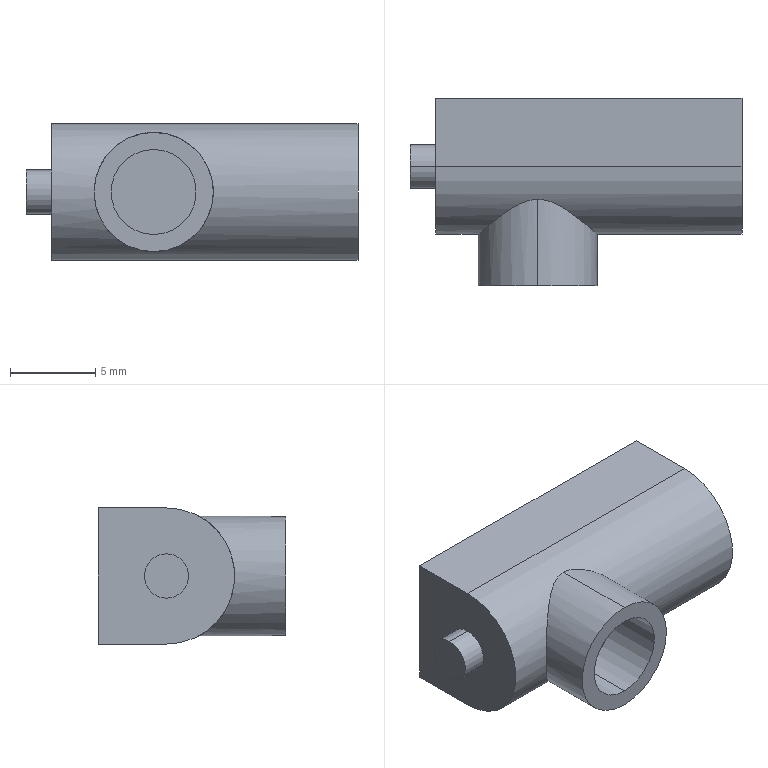Part | STEP file | _AF30-A(0)_DRAIN | 1 solid | 15 faces | box 19.5 x 11 x 8 mm | volume 1100 mm3 | plane 8 | cylinder 7 | commonest cylinder face diameters 2.6 x2 5 x2 7 x2 8 x1
STEP:
#1=CARTESIAN_POINT('',(-3.,-5.936,3.5));
#2=VERTEX_POINT('',#1);
#3=CARTESIAN_POINT('',(-3.,-5.936,-3.5));
#4=VERTEX_POINT('',#3);
#5=CARTESIAN_POINT('',(-3.,-5.936,3.5));
#6=CARTESIAN_POINT('',(-2.749,-5.936,3.5));
#7=CARTESIAN_POINT('',(-2.506,-5.987,3.473));
#8=CARTESIAN_POINT('',(-2.044,-6.149,3.375));
#9=CARTESIAN_POINT('',(-1.832,-6.255,3.307));
#10=CARTESIAN_POINT('',(-1.429,-6.488,3.135));
#11=CARTESIAN_POINT('',(-1.239,-6.614,3.032));
#12=CARTESIAN_POINT('',(-0.8863,-6.864,2.798));
#13=CARTESIAN_POINT('',(-0.7211,-6.989,2.665));
#14=CARTESIAN_POINT('',(-0.4112,-7.232,2.365));
#15=CARTESIAN_POINT('',(-0.2667,-7.349,2.197));
#16=CARTESIAN_POINT('',(-0.01033,-7.561,1.833));
#17=CARTESIAN_POINT('',(0.1034,-7.658,1.635));
#18=CARTESIAN_POINT('',(0.2947,-7.821,1.204));
#19=CARTESIAN_POINT('',(0.3694,-7.886,0.9781));
#20=CARTESIAN_POINT('',(0.4467,-7.953,0.6204));
#21=CARTESIAN_POINT('',(0.4667,-7.971,0.4973));
#22=CARTESIAN_POINT('',(0.4931,-7.994,0.2519));
#23=CARTESIAN_POINT('',(0.4998,-8.,0.1289));
#24=CARTESIAN_POINT('',(0.5004,-8.,-0.2405));
#25=CARTESIAN_POINT('',(0.4739,-7.977,-0.4912));
#26=CARTESIAN_POINT('',(0.3724,-7.889,-0.9675));
#27=CARTESIAN_POINT('',(0.2971,-7.823,-1.198));
#28=CARTESIAN_POINT('',(0.01254,-7.58,-1.843));
#29=CARTESIAN_POINT('',(-0.2533,-7.355,-2.211));
#30=CARTESIAN_POINT('',(-0.7151,-6.994,-2.66));
#31=CARTESIAN_POINT('',(-0.8806,-6.868,-2.794));
#32=CARTESIAN_POINT('',(-1.238,-6.615,-3.032));
#33=CARTESIAN_POINT('',(-1.426,-6.49,-3.134));
#34=CARTESIAN_POINT('',(-1.726,-6.316,-3.262));
#35=CARTESIAN_POINT('',(-1.83,-6.261,-3.301));
#36=CARTESIAN_POINT('',(-2.045,-6.157,-3.369));
#37=CARTESIAN_POINT('',(-2.158,-6.109,-3.399));
#38=CARTESIAN_POINT('',(-2.387,-6.028,-3.448));
#39=CARTESIAN_POINT('',(-2.505,-5.995,-3.467));
#40=CARTESIAN_POINT('',(-2.749,-5.949,-3.493));
#41=CARTESIAN_POINT('',(-2.874,-5.936,-3.5));
#42=CARTESIAN_POINT('',(-3.,-5.936,-3.5));
#43=B_SPLINE_CURVE_WITH_KNOTS('',3,(#5,#6,#7,#8,#9,#10,#11,#12,#13,#14,#15,#16,#17,#18,#19,#20,#21,#22,#23,#24,#25,#26,#27,#28,#29,#30,#31,#32,#33,#34,#35,#36,#37,#38,#39,#40,#41,#42),.UNSPECIFIED.,.F.,.F.,(4,2,2,2,2,2,2,2,2,2,2,2,2,2,2,2,2,2,4),(0.01185,0.0126,0.01334,0.01408,0.01482,0.01556,0.0163,0.01704,0.01741,0.01778,0.01852,0.01927,0.02075,0.02149,0.02223,0.0226,0.02297,0.02334,0.02371),.UNSPECIFIED.);
#44=EDGE_CURVE('',#2,#4,#43,.T.);
#45=ORIENTED_EDGE('',*,*,#44,.F.);
#46=CARTESIAN_POINT('',(-3.,-11.,3.5));
#47=VERTEX_POINT('',#46);
#48=CARTESIAN_POINT('',(-3.,0.,3.5));
#49=DIRECTION('',(0.,-1.,0.));
#50=VECTOR('',#49,1000.);
#51=LINE('',#48,#50);
#52=EDGE_CURVE('',#2,#47,#51,.T.);
#53=ORIENTED_EDGE('',*,*,#52,.T.);
#54=CARTESIAN_POINT('',(-3.,-11.,-3.5));
#55=VERTEX_POINT('',#54);
#56=CARTESIAN_POINT('',(-3.,-11.,0.));
#57=DIRECTION('',(0.,1.,0.));
#58=DIRECTION('',(0.,0.,-1.));
#59=AXIS2_PLACEMENT_3D('',#56,#57,#58);
#60=CIRCLE('',#59,3.5);
#61=EDGE_CURVE('',#47,#55,#60,.T.);
#62=ORIENTED_EDGE('',*,*,#61,.T.);
#63=CARTESIAN_POINT('',(-3.,0.,-3.5));
#64=DIRECTION('',(0.,-1.,0.));
#65=VECTOR('',#64,1000.);
#66=LINE('',#63,#65);
#67=EDGE_CURVE('',#4,#55,#66,.T.);
#68=ORIENTED_EDGE('',*,*,#67,.F.);
#69=EDGE_LOOP('',(#45,#53,#62,#68));
#70=FACE_OUTER_BOUND('',#69,.T.);
#71=CARTESIAN_POINT('',(-3.,0.,0.));
#72=DIRECTION('',(0.,-1.,0.));
#73=DIRECTION('',(0.,0.,-1.));
#74=AXIS2_PLACEMENT_3D('',#71,#72,#73);
#75=CYLINDRICAL_SURFACE('',#74,3.5);
#76=ADVANCED_FACE('',(#70),#75,.T.);
#77=CARTESIAN_POINT('',(-10.5,-4.,-1.3));
#78=VERTEX_POINT('',#77);
#79=CARTESIAN_POINT('',(-10.5,-4.,1.3));
#80=VERTEX_POINT('',#79);
#81=CARTESIAN_POINT('',(-10.5,-4.,0.));
#82=DIRECTION('',(1.,0.,0.));
#83=DIRECTION('',(0.,0.,-1.));
#84=AXIS2_PLACEMENT_3D('',#81,#82,#83);
#85=CIRCLE('',#84,1.3);
#86=EDGE_CURVE('',#78,#80,#85,.T.);
#87=ORIENTED_EDGE('',*,*,#86,.T.);
#88=CARTESIAN_POINT('',(-9.,-4.,1.3));
#89=VERTEX_POINT('',#88);
#90=CARTESIAN_POINT('',(-10.5,-4.,1.3));
#91=DIRECTION('',(1.,0.,0.));
#92=VECTOR('',#91,1000.);
#93=LINE('',#90,#92);
#94=EDGE_CURVE('',#80,#89,#93,.T.);
#95=ORIENTED_EDGE('',*,*,#94,.T.);
#96=CARTESIAN_POINT('',(-9.,-4.,-1.3));
#97=VERTEX_POINT('',#96);
#98=CARTESIAN_POINT('',(-9.,-4.,0.));
#99=DIRECTION('',(-1.,0.,0.));
#100=DIRECTION('',(0.,0.,-1.));
#101=AXIS2_PLACEMENT_3D('',#98,#99,#100);
#102=CIRCLE('',#101,1.3);
#103=EDGE_CURVE('',#89,#97,#102,.T.);
#104=ORIENTED_EDGE('',*,*,#103,.T.);
#105=CARTESIAN_POINT('',(-10.5,-4.,-1.3));
#106=DIRECTION('',(1.,0.,0.));
#107=VECTOR('',#106,1000.);
#108=LINE('',#105,#107);
#109=EDGE_CURVE('',#78,#97,#108,.T.);
#110=ORIENTED_EDGE('',*,*,#109,.F.);
#111=EDGE_LOOP('',(#87,#95,#104,#110));
#112=FACE_OUTER_BOUND('',#111,.T.);
#113=CARTESIAN_POINT('',(-10.5,-4.,0.));
#114=DIRECTION('',(1.,0.,0.));
#115=DIRECTION('',(0.,0.,-1.));
#116=AXIS2_PLACEMENT_3D('',#113,#114,#115);
#117=CYLINDRICAL_SURFACE('',#116,1.3);
#118=ADVANCED_FACE('',(#112),#117,.T.);
#119=CARTESIAN_POINT('',(-3.,-11.,2.5));
#120=VERTEX_POINT('',#119);
#121=CARTESIAN_POINT('',(-3.,-11.,-2.5));
#122=VERTEX_POINT('',#121);
#123=CARTESIAN_POINT('',(-3.,-11.,0.));
#124=DIRECTION('',(0.,-1.,0.));
#125=DIRECTION('',(0.,0.,1.));
#126=AXIS2_PLACEMENT_3D('',#123,#124,#125);
#127=CIRCLE('',#126,2.5);
#128=EDGE_CURVE('',#120,#122,#127,.T.);
#129=ORIENTED_EDGE('',*,*,#128,.T.);
#130=CARTESIAN_POINT('',(-3.,-7.5,-2.5));
#131=VERTEX_POINT('',#130);
#132=CARTESIAN_POINT('',(-3.,-7.5,-2.5));
#133=DIRECTION('',(0.,1.,0.));
#134=VECTOR('',#133,1000.);
#135=LINE('',#132,#134);
#136=EDGE_CURVE('',#122,#131,#135,.T.);
#137=ORIENTED_EDGE('',*,*,#136,.T.);
#138=CARTESIAN_POINT('',(-3.,-7.5,2.5));
#139=VERTEX_POINT('',#138);
#140=CARTESIAN_POINT('',(-3.,-7.5,0.));
#141=DIRECTION('',(0.,-1.,0.));
#142=DIRECTION('',(0.,0.,1.));
#143=AXIS2_PLACEMENT_3D('',#140,#141,#142);
#144=CIRCLE('',#143,2.5);
#145=EDGE_CURVE('',#139,#131,#144,.T.);
#146=ORIENTED_EDGE('',*,*,#145,.F.);
#147=CARTESIAN_POINT('',(-3.,-7.5,2.5));
#148=DIRECTION('',(0.,1.,0.));
#149=VECTOR('',#148,1000.);
#150=LINE('',#147,#149);
#151=EDGE_CURVE('',#120,#139,#150,.T.);
#152=ORIENTED_EDGE('',*,*,#151,.F.);
#153=EDGE_LOOP('',(#129,#137,#146,#152));
#154=FACE_OUTER_BOUND('',#153,.T.);
#155=CARTESIAN_POINT('',(-3.,-7.5,0.));
#156=DIRECTION('',(0.,1.,0.));
#157=DIRECTION('',(0.,0.,1.));
#158=AXIS2_PLACEMENT_3D('',#155,#156,#157);
#159=CYLINDRICAL_SURFACE('',#158,2.5);
#160=ADVANCED_FACE('',(#154),#159,.F.);
#161=CARTESIAN_POINT('',(-9.,-4.,4.));
#162=VERTEX_POINT('',#161);
#163=CARTESIAN_POINT('',(-9.,-4.,-4.));
#164=VERTEX_POINT('',#163);
#165=CARTESIAN_POINT('',(-9.,-4.,0.));
#166=DIRECTION('',(1.,0.,0.));
#167=DIRECTION('',(0.,0.,-1.));
#168=AXIS2_PLACEMENT_3D('',#165,#166,#167);
#169=CIRCLE('',#168,4.);
#170=EDGE_CURVE('',#162,#164,#169,.T.);
#171=ORIENTED_EDGE('',*,*,#170,.T.);
#172=CARTESIAN_POINT('',(9.,-4.,-4.));
#173=VERTEX_POINT('',#172);
#174=CARTESIAN_POINT('',(9.,-4.,-4.));
#175=DIRECTION('',(1.,0.,0.));
#176=VECTOR('',#175,1000.);
#177=LINE('',#174,#176);
#178=EDGE_CURVE('',#164,#173,#177,.T.);
#179=ORIENTED_EDGE('',*,*,#178,.T.);
#180=CARTESIAN_POINT('',(9.,-4.,4.));
#181=VERTEX_POINT('',#180);
#182=CARTESIAN_POINT('',(9.,-4.,0.));
#183=DIRECTION('',(-1.,0.,0.));
#184=DIRECTION('',(0.,0.,-1.));
#185=AXIS2_PLACEMENT_3D('',#182,#183,#184);
#186=CIRCLE('',#185,4.);
#187=EDGE_CURVE('',#173,#181,#186,.T.);
#188=ORIENTED_EDGE('',*,*,#187,.T.);
#189=CARTESIAN_POINT('',(9.,-4.,4.));
#190=DIRECTION('',(-1.,0.,0.));
#191=VECTOR('',#190,1000.);
#192=LINE('',#189,#191);
#193=EDGE_CURVE('',#181,#162,#192,.T.);
#194=ORIENTED_EDGE('',*,*,#193,.T.);
#195=EDGE_LOOP('',(#171,#179,#188,#194));
#196=FACE_OUTER_BOUND('',#195,.T.);
#197=CARTESIAN_POINT('',(-3.,-5.936,-3.5));
#198=CARTESIAN_POINT('',(-3.251,-5.936,-3.5));
#199=CARTESIAN_POINT('',(-3.494,-5.987,-3.473));
#200=CARTESIAN_POINT('',(-3.956,-6.149,-3.375));
#201=CARTESIAN_POINT('',(-4.168,-6.255,-3.307));
#202=CARTESIAN_POINT('',(-4.571,-6.488,-3.135));
#203=CARTESIAN_POINT('',(-4.761,-6.614,-3.032));
#204=CARTESIAN_POINT('',(-5.114,-6.864,-2.798));
#205=CARTESIAN_POINT('',(-5.279,-6.989,-2.665));
#206=CARTESIAN_POINT('',(-5.589,-7.232,-2.365));
#207=CARTESIAN_POINT('',(-5.733,-7.349,-2.197));
#208=CARTESIAN_POINT('',(-5.99,-7.561,-1.833));
#209=CARTESIAN_POINT('',(-6.103,-7.658,-1.635));
#210=CARTESIAN_POINT('',(-6.295,-7.821,-1.204));
#211=CARTESIAN_POINT('',(-6.369,-7.886,-0.9781));
#212=CARTESIAN_POINT('',(-6.447,-7.953,-0.6204));
#213=CARTESIAN_POINT('',(-6.467,-7.971,-0.4973));
#214=CARTESIAN_POINT('',(-6.493,-7.994,-0.2519));
#215=CARTESIAN_POINT('',(-6.5,-8.,-0.1289));
#216=CARTESIAN_POINT('',(-6.5,-8.,0.2405));
#217=CARTESIAN_POINT('',(-6.474,-7.977,0.4912));
#218=CARTESIAN_POINT('',(-6.372,-7.889,0.9675));
#219=CARTESIAN_POINT('',(-6.297,-7.823,1.198));
#220=CARTESIAN_POINT('',(-6.013,-7.58,1.843));
#221=CARTESIAN_POINT('',(-5.747,-7.355,2.211));
#222=CARTESIAN_POINT('',(-5.285,-6.994,2.66));
#223=CARTESIAN_POINT('',(-5.119,-6.868,2.794));
#224=CARTESIAN_POINT('',(-4.762,-6.615,3.032));
#225=CARTESIAN_POINT('',(-4.574,-6.49,3.134));
#226=CARTESIAN_POINT('',(-4.274,-6.316,3.262));
#227=CARTESIAN_POINT('',(-4.17,-6.261,3.301));
#228=CARTESIAN_POINT('',(-3.955,-6.157,3.369));
#229=CARTESIAN_POINT('',(-3.842,-6.109,3.399));
#230=CARTESIAN_POINT('',(-3.613,-6.028,3.448));
#231=CARTESIAN_POINT('',(-3.495,-5.995,3.467));
#232=CARTESIAN_POINT('',(-3.251,-5.949,3.493));
#233=CARTESIAN_POINT('',(-3.126,-5.936,3.5));
#234=CARTESIAN_POINT('',(-3.,-5.936,3.5));
#235=B_SPLINE_CURVE_WITH_KNOTS('',3,(#197,#198,#199,#200,#201,#202,#203,#204,#205,#206,#207,#208,#209,#210,#211,#212,#213,#214,#215,#216,#217,#218,#219,#220,#221,#222,#223,#224,#225,#226,#227,#228,#229,#230,#231,#232,#233,#234),.UNSPECIFIED.,.F.,.F.,(4,2,2,2,2,2,2,2,2,2,2,2,2,2,2,2,2,2,4),(0.,0.0007409,0.001482,0.002223,0.002964,0.003705,0.004445,0.005186,0.005557,0.005927,0.006668,0.007409,0.008891,0.009632,0.01037,0.01074,0.01111,0.01148,0.01185),.UNSPECIFIED.);
#236=EDGE_CURVE('',#4,#2,#235,.T.);
#237=ORIENTED_EDGE('',*,*,#236,.T.);
#238=ORIENTED_EDGE('',*,*,#44,.T.);
#239=EDGE_LOOP('',(#237,#238));
#240=FACE_BOUND('',#239,.T.);
#241=CARTESIAN_POINT('',(9.,-4.,0.));
#242=DIRECTION('',(1.,0.,0.));
#243=DIRECTION('',(0.,0.,-1.));
#244=AXIS2_PLACEMENT_3D('',#241,#242,#243);
#245=CYLINDRICAL_SURFACE('',#244,4.);
#246=ADVANCED_FACE('',(#196,#240),#245,.T.);
#247=CARTESIAN_POINT('',(9.,0.,-4.));
#248=VERTEX_POINT('',#247);
#249=CARTESIAN_POINT('',(9.,-4.,-4.));
#250=DIRECTION('',(0.,1.,0.));
#251=VECTOR('',#250,1000.);
#252=LINE('',#249,#251);
#253=EDGE_CURVE('',#173,#248,#252,.T.);
#254=ORIENTED_EDGE('',*,*,#253,.F.);
#255=ORIENTED_EDGE('',*,*,#178,.F.);
#256=CARTESIAN_POINT('',(-9.,0.,-4.));
#257=VERTEX_POINT('',#256);
#258=CARTESIAN_POINT('',(-9.,-4.,-4.));
#259=DIRECTION('',(0.,-1.,0.));
#260=VECTOR('',#259,1000.);
#261=LINE('',#258,#260);
#262=EDGE_CURVE('',#257,#164,#261,.T.);
#263=ORIENTED_EDGE('',*,*,#262,.F.);
#264=CARTESIAN_POINT('',(9.,0.,-4.));
#265=DIRECTION('',(-1.,0.,0.));
#266=VECTOR('',#265,1000.);
#267=LINE('',#264,#266);
#268=EDGE_CURVE('',#248,#257,#267,.T.);
#269=ORIENTED_EDGE('',*,*,#268,.F.);
#270=EDGE_LOOP('',(#254,#255,#263,#269));
#271=FACE_OUTER_BOUND('',#270,.T.);
#272=CARTESIAN_POINT('',(9.,-4.,-4.));
#273=DIRECTION('',(0.,0.,1.));
#274=DIRECTION('',(1.,0.,0.));
#275=AXIS2_PLACEMENT_3D('',#272,#273,#274);
#276=PLANE('',#275);
#277=ADVANCED_FACE('',(#271),#276,.F.);
#278=CARTESIAN_POINT('',(-9.,-4.,0.));
#279=DIRECTION('',(-1.,0.,0.));
#280=DIRECTION('',(0.,0.,-1.));
#281=AXIS2_PLACEMENT_3D('',#278,#279,#280);
#282=CIRCLE('',#281,1.3);
#283=EDGE_CURVE('',#97,#89,#282,.T.);
#284=ORIENTED_EDGE('',*,*,#283,.F.);
#285=ORIENTED_EDGE('',*,*,#103,.F.);
#286=EDGE_LOOP('',(#284,#285));
#287=FACE_BOUND('',#286,.T.);
#288=ORIENTED_EDGE('',*,*,#262,.T.);
#289=ORIENTED_EDGE('',*,*,#170,.F.);
#290=CARTESIAN_POINT('',(-9.,0.,4.));
#291=VERTEX_POINT('',#290);
#292=CARTESIAN_POINT('',(-9.,-4.,4.));
#293=DIRECTION('',(0.,-1.,0.));
#294=VECTOR('',#293,1000.);
#295=LINE('',#292,#294);
#296=EDGE_CURVE('',#291,#162,#295,.T.);
#297=ORIENTED_EDGE('',*,*,#296,.F.);
#298=CARTESIAN_POINT('',(-9.,0.,0.));
#299=DIRECTION('',(0.,0.,1.));
#300=VECTOR('',#299,1000.);
#301=LINE('',#298,#300);
#302=EDGE_CURVE('',#257,#291,#301,.T.);
#303=ORIENTED_EDGE('',*,*,#302,.F.);
#304=EDGE_LOOP('',(#288,#289,#297,#303));
#305=FACE_OUTER_BOUND('',#304,.T.);
#306=CARTESIAN_POINT('',(-9.,-4.,0.));
#307=DIRECTION('',(1.,0.,0.));
#308=DIRECTION('',(0.,0.,-1.));
#309=AXIS2_PLACEMENT_3D('',#306,#307,#308);
#310=PLANE('',#309);
#311=ADVANCED_FACE('',(#287,#305),#310,.F.);
#312=CARTESIAN_POINT('',(9.,0.,4.));
#313=VERTEX_POINT('',#312);
#314=CARTESIAN_POINT('',(9.,0.,4.));
#315=DIRECTION('',(0.,-1.,0.));
#316=VECTOR('',#315,1000.);
#317=LINE('',#314,#316);
#318=EDGE_CURVE('',#313,#181,#317,.T.);
#319=ORIENTED_EDGE('',*,*,#318,.F.);
#320=CARTESIAN_POINT('',(9.,0.,4.));
#321=DIRECTION('',(1.,0.,0.));
#322=VECTOR('',#321,1000.);
#323=LINE('',#320,#322);
#324=EDGE_CURVE('',#291,#313,#323,.T.);
#325=ORIENTED_EDGE('',*,*,#324,.F.);
#326=ORIENTED_EDGE('',*,*,#296,.T.);
#327=ORIENTED_EDGE('',*,*,#193,.F.);
#328=EDGE_LOOP('',(#319,#325,#326,#327));
#329=FACE_OUTER_BOUND('',#328,.T.);
#330=CARTESIAN_POINT('',(9.,0.,4.));
#331=DIRECTION('',(0.,0.,-1.));
#332=DIRECTION('',(-1.,0.,0.));
#333=AXIS2_PLACEMENT_3D('',#330,#331,#332);
#334=PLANE('',#333);
#335=ADVANCED_FACE('',(#329),#334,.F.);
#336=ORIENTED_EDGE('',*,*,#318,.T.);
#337=ORIENTED_EDGE('',*,*,#187,.F.);
#338=ORIENTED_EDGE('',*,*,#253,.T.);
#339=CARTESIAN_POINT('',(9.,0.,0.));
#340=DIRECTION('',(0.,0.,1.));
#341=VECTOR('',#340,1000.);
#342=LINE('',#339,#341);
#343=EDGE_CURVE('',#248,#313,#342,.T.);
#344=ORIENTED_EDGE('',*,*,#343,.T.);
#345=EDGE_LOOP('',(#336,#337,#338,#344));
#346=FACE_OUTER_BOUND('',#345,.T.);
#347=CARTESIAN_POINT('',(9.,-4.,0.));
#348=DIRECTION('',(1.,0.,0.));
#349=DIRECTION('',(0.,0.,-1.));
#350=AXIS2_PLACEMENT_3D('',#347,#348,#349);
#351=PLANE('',#350);
#352=ADVANCED_FACE('',(#346),#351,.T.);
#353=ORIENTED_EDGE('',*,*,#52,.F.);
#354=ORIENTED_EDGE('',*,*,#236,.F.);
#355=ORIENTED_EDGE('',*,*,#67,.T.);
#356=CARTESIAN_POINT('',(-3.,-11.,0.));
#357=DIRECTION('',(0.,1.,0.));
#358=DIRECTION('',(0.,0.,-1.));
#359=AXIS2_PLACEMENT_3D('',#356,#357,#358);
#360=CIRCLE('',#359,3.5);
#361=EDGE_CURVE('',#55,#47,#360,.T.);
#362=ORIENTED_EDGE('',*,*,#361,.T.);
#363=EDGE_LOOP('',(#353,#354,#355,#362));
#364=FACE_OUTER_BOUND('',#363,.T.);
#365=CARTESIAN_POINT('',(-3.,0.,0.));
#366=DIRECTION('',(0.,-1.,0.));
#367=DIRECTION('',(0.,0.,-1.));
#368=AXIS2_PLACEMENT_3D('',#365,#366,#367);
#369=CYLINDRICAL_SURFACE('',#368,3.5);
#370=ADVANCED_FACE('',(#364),#369,.T.);
#371=ORIENTED_EDGE('',*,*,#343,.F.);
#372=ORIENTED_EDGE('',*,*,#268,.T.);
#373=ORIENTED_EDGE('',*,*,#302,.T.);
#374=ORIENTED_EDGE('',*,*,#324,.T.);
#375=EDGE_LOOP('',(#371,#372,#373,#374));
#376=FACE_OUTER_BOUND('',#375,.T.);
#377=CARTESIAN_POINT('',(9.,0.,-4.));
#378=DIRECTION('',(0.,-1.,0.));
#379=DIRECTION('',(0.,0.,-1.));
#380=AXIS2_PLACEMENT_3D('',#377,#378,#379);
#381=PLANE('',#380);
#382=ADVANCED_FACE('',(#376),#381,.F.);
#383=ORIENTED_EDGE('',*,*,#94,.F.);
#384=CARTESIAN_POINT('',(-10.5,-4.,0.));
#385=DIRECTION('',(1.,0.,0.));
#386=DIRECTION('',(0.,0.,-1.));
#387=AXIS2_PLACEMENT_3D('',#384,#385,#386);
#388=CIRCLE('',#387,1.3);
#389=EDGE_CURVE('',#80,#78,#388,.T.);
#390=ORIENTED_EDGE('',*,*,#389,.T.);
#391=ORIENTED_EDGE('',*,*,#109,.T.);
#392=ORIENTED_EDGE('',*,*,#283,.T.);
#393=EDGE_LOOP('',(#383,#390,#391,#392));
#394=FACE_OUTER_BOUND('',#393,.T.);
#395=CARTESIAN_POINT('',(-10.5,-4.,0.));
#396=DIRECTION('',(1.,0.,0.));
#397=DIRECTION('',(0.,0.,-1.));
#398=AXIS2_PLACEMENT_3D('',#395,#396,#397);
#399=CYLINDRICAL_SURFACE('',#398,1.3);
#400=ADVANCED_FACE('',(#394),#399,.T.);
#401=ORIENTED_EDGE('',*,*,#361,.F.);
#402=ORIENTED_EDGE('',*,*,#61,.F.);
#403=EDGE_LOOP('',(#401,#402));
#404=FACE_OUTER_BOUND('',#403,.T.);
#405=ORIENTED_EDGE('',*,*,#128,.F.);
#406=CARTESIAN_POINT('',(-3.,-11.,0.));
#407=DIRECTION('',(0.,-1.,0.));
#408=DIRECTION('',(0.,0.,1.));
#409=AXIS2_PLACEMENT_3D('',#406,#407,#408);
#410=CIRCLE('',#409,2.5);
#411=EDGE_CURVE('',#122,#120,#410,.T.);
#412=ORIENTED_EDGE('',*,*,#411,.F.);
#413=EDGE_LOOP('',(#405,#412));
#414=FACE_BOUND('',#413,.T.);
#415=CARTESIAN_POINT('',(-3.,-11.,0.));
#416=DIRECTION('',(0.,1.,0.));
#417=DIRECTION('',(0.,0.,1.));
#418=AXIS2_PLACEMENT_3D('',#415,#416,#417);
#419=PLANE('',#418);
#420=ADVANCED_FACE('',(#404,#414),#419,.F.);
#421=ORIENTED_EDGE('',*,*,#86,.F.);
#422=ORIENTED_EDGE('',*,*,#389,.F.);
#423=EDGE_LOOP('',(#421,#422));
#424=FACE_OUTER_BOUND('',#423,.T.);
#425=CARTESIAN_POINT('',(-10.5,-5.3,0.));
#426=DIRECTION('',(1.,0.,0.));
#427=DIRECTION('',(0.,0.,-1.));
#428=AXIS2_PLACEMENT_3D('',#425,#426,#427);
#429=PLANE('',#428);
#430=ADVANCED_FACE('',(#424),#429,.F.);
#431=ORIENTED_EDGE('',*,*,#136,.F.);
#432=ORIENTED_EDGE('',*,*,#411,.T.);
#433=ORIENTED_EDGE('',*,*,#151,.T.);
#434=CARTESIAN_POINT('',(-3.,-7.5,0.));
#435=DIRECTION('',(0.,-1.,0.));
#436=DIRECTION('',(0.,0.,1.));
#437=AXIS2_PLACEMENT_3D('',#434,#435,#436);
#438=CIRCLE('',#437,2.5);
#439=EDGE_CURVE('',#131,#139,#438,.T.);
#440=ORIENTED_EDGE('',*,*,#439,.F.);
#441=EDGE_LOOP('',(#431,#432,#433,#440));
#442=FACE_OUTER_BOUND('',#441,.T.);
#443=CARTESIAN_POINT('',(-3.,-7.5,0.));
#444=DIRECTION('',(0.,1.,0.));
#445=DIRECTION('',(0.,0.,1.));
#446=AXIS2_PLACEMENT_3D('',#443,#444,#445);
#447=CYLINDRICAL_SURFACE('',#446,2.5);
#448=ADVANCED_FACE('',(#442),#447,.F.);
#449=ORIENTED_EDGE('',*,*,#145,.T.);
#450=ORIENTED_EDGE('',*,*,#439,.T.);
#451=EDGE_LOOP('',(#449,#450));
#452=FACE_OUTER_BOUND('',#451,.T.);
#453=CARTESIAN_POINT('',(-3.,-7.5,0.));
#454=DIRECTION('',(0.,-1.,0.));
#455=DIRECTION('',(0.,0.,-1.));
#456=AXIS2_PLACEMENT_3D('',#453,#454,#455);
#457=PLANE('',#456);
#458=ADVANCED_FACE('',(#452),#457,.T.);
#459=CLOSED_SHELL('',(#76,#118,#160,#246,#277,#311,#335,#352,#370,#382,#400,#420,#430,#448,#458));
#460=MANIFOLD_SOLID_BREP('',#459);
#461=CARTESIAN_POINT('',(0.,0.,0.));
#462=DIRECTION('',(0.,0.,1.));
#463=DIRECTION('',(1.,0.,0.));
#464=AXIS2_PLACEMENT_3D('',#461,#462,#463);
#465=(LENGTH_UNIT()NAMED_UNIT(*)SI_UNIT(.MILLI.,.METRE.));
#466=UNCERTAINTY_MEASURE_WITH_UNIT(LENGTH_MEASURE(0.00001),#465,'','');
#467=(NAMED_UNIT(*)PLANE_ANGLE_UNIT()SI_UNIT($,.RADIAN.));
#468=(NAMED_UNIT(*)SI_UNIT($,.STERADIAN.)SOLID_ANGLE_UNIT());
#469=(GEOMETRIC_REPRESENTATION_CONTEXT(3)GLOBAL_UNCERTAINTY_ASSIGNED_CONTEXT((#466))GLOBAL_UNIT_ASSIGNED_CONTEXT((#465,#467,#468))REPRESENTATION_CONTEXT('',''));
#470=ADVANCED_BREP_SHAPE_REPRESENTATION('',(#460,#464),#469);